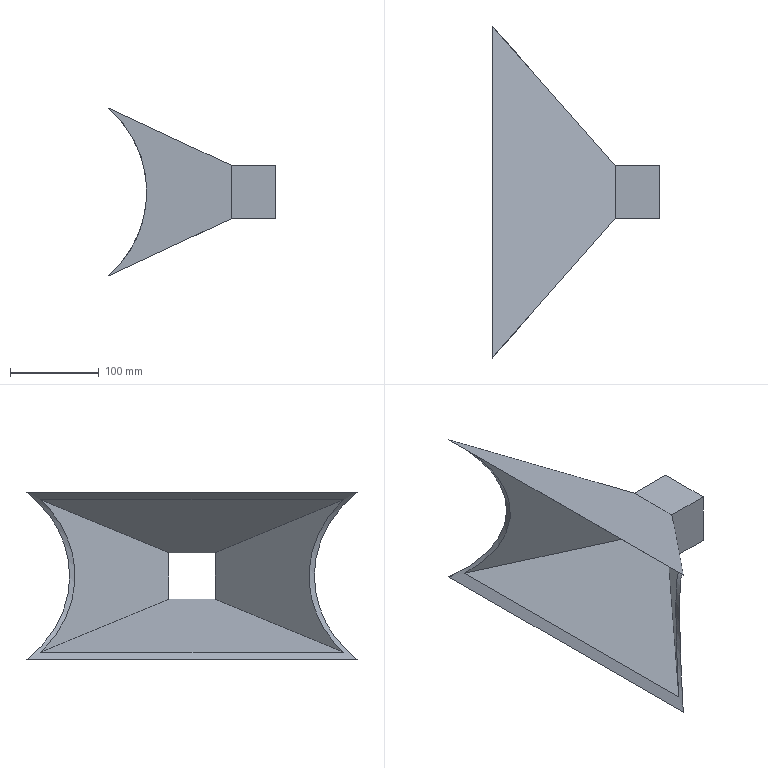Part | NX | features NSIDED_SURFACE 6, DATUM_CSYS 5, LINE 4, SKETCH 3, EXTRUDE 2, SEW 1, SHELL 1 | 1 solid | 18 faces | box 188.137 x 373.11 x 188.928 mm | volume 418507 mm3 | spline 9 | plane 8 | cylinder 1 | commonest cylinder face diameters 250 x1
STEP:
#1=CARTESIAN_POINT('',(11.863,-186.555,94.464));
#2=VERTEX_POINT('',#1);
#3=CARTESIAN_POINT('',(11.863,186.555,94.464));
#4=VERTEX_POINT('',#3);
#5=CARTESIAN_POINT('',(11.863,-186.555,94.464));
#6=CARTESIAN_POINT('',(11.863,-62.185,94.464));
#7=CARTESIAN_POINT('',(11.863,62.185,94.464));
#8=CARTESIAN_POINT('',(11.863,186.555,94.464));
#9=B_SPLINE_CURVE_WITH_KNOTS('',3,(#5,#6,#7,#8),.UNSPECIFIED.,.F.,.F.,(4,4),(0.02059,0.3937),.UNSPECIFIED.);
#10=EDGE_CURVE('',#2,#4,#9,.T.);
#11=ORIENTED_EDGE('',*,*,#10,.F.);
#12=CARTESIAN_POINT('',(150.,-30.,30.));
#13=VERTEX_POINT('',#12);
#14=CARTESIAN_POINT('',(150.,-30.,30.));
#15=CARTESIAN_POINT('',(103.954,-82.185,51.488));
#16=CARTESIAN_POINT('',(57.909,-134.37,72.976));
#17=CARTESIAN_POINT('',(11.863,-186.555,94.464));
#18=B_SPLINE_CURVE_WITH_KNOTS('',3,(#14,#15,#16,#17),.UNSPECIFIED.,.F.,.F.,(4,4),(0.,0.9209),.UNSPECIFIED.);
#19=EDGE_CURVE('',#2,#13,#18,.F.);
#20=ORIENTED_EDGE('',*,*,#19,.T.);
#21=CARTESIAN_POINT('',(150.,30.,30.));
#22=VERTEX_POINT('',#21);
#23=CARTESIAN_POINT('',(150.,-30.,30.));
#24=CARTESIAN_POINT('',(150.,-10.,30.));
#25=CARTESIAN_POINT('',(150.,10.,30.));
#26=CARTESIAN_POINT('',(150.,30.,30.));
#27=B_SPLINE_CURVE_WITH_KNOTS('',3,(#23,#24,#25,#26),.UNSPECIFIED.,.F.,.F.,(4,4),(0.,1.),.UNSPECIFIED.);
#28=EDGE_CURVE('',#22,#13,#27,.F.);
#29=ORIENTED_EDGE('',*,*,#28,.F.);
#30=CARTESIAN_POINT('',(11.863,186.555,94.464));
#31=CARTESIAN_POINT('',(57.909,134.37,72.976));
#32=CARTESIAN_POINT('',(103.954,82.185,51.488));
#33=CARTESIAN_POINT('',(150.,30.,30.));
#34=B_SPLINE_CURVE_WITH_KNOTS('',3,(#30,#31,#32,#33),.UNSPECIFIED.,.F.,.F.,(4,4),(0.07909,1.),.UNSPECIFIED.);
#35=EDGE_CURVE('',#22,#4,#34,.F.);
#36=ORIENTED_EDGE('',*,*,#35,.T.);
#37=EDGE_LOOP('',(#11,#20,#29,#36));
#38=FACE_BOUND('',#37,.T.);
#39=CARTESIAN_POINT('',(198.589,114.103,7.325));
#40=CARTESIAN_POINT('',(136.194,139.062,36.443));
#41=CARTESIAN_POINT('',(73.799,164.02,65.561));
#42=CARTESIAN_POINT('',(11.403,188.978,94.678));
#43=CARTESIAN_POINT('',(162.048,2.857,24.378));
#44=CARTESIAN_POINT('',(99.653,27.815,53.495));
#45=CARTESIAN_POINT('',(37.258,52.773,82.613));
#46=CARTESIAN_POINT('',(-25.137,77.731,111.731));
#47=CARTESIAN_POINT('',(125.507,-108.389,41.43));
#48=CARTESIAN_POINT('',(63.112,-83.431,70.548));
#49=CARTESIAN_POINT('',(0.7171,-58.473,99.665));
#50=CARTESIAN_POINT('',(-61.678,-33.515,128.783));
#51=CARTESIAN_POINT('',(88.967,-219.635,58.482));
#52=CARTESIAN_POINT('',(26.572,-194.677,87.6));
#53=CARTESIAN_POINT('',(-35.824,-169.719,116.718));
#54=CARTESIAN_POINT('',(-98.219,-144.761,145.835));
#55=B_SPLINE_SURFACE_WITH_KNOTS('',3,3,((#39,#40,#41,#42),(#43,#44,#45,#46),(#47,#48,#49,#50),(#51,#52,#53,#54)),.PLANE_SURF.,.F.,.F.,.F.,(4,4),(4,4),(0.06014,0.9183),(0.04039,0.894),.PIECEWISE_BEZIER_KNOTS.);
#56=ADVANCED_FACE('',(#38),#55,.F.);
#57=CARTESIAN_POINT('',(11.863,186.555,-94.464));
#58=VERTEX_POINT('',#57);
#59=CARTESIAN_POINT('',(150.,30.,-30.));
#60=VERTEX_POINT('',#59);
#61=CARTESIAN_POINT('',(150.,30.,-30.));
#62=CARTESIAN_POINT('',(103.954,82.185,-51.488));
#63=CARTESIAN_POINT('',(57.909,134.37,-72.976));
#64=CARTESIAN_POINT('',(11.863,186.555,-94.464));
#65=B_SPLINE_CURVE_WITH_KNOTS('',3,(#61,#62,#63,#64),.UNSPECIFIED.,.F.,.F.,(4,4),(0.,0.9209),.UNSPECIFIED.);
#66=EDGE_CURVE('',#58,#60,#65,.F.);
#67=ORIENTED_EDGE('',*,*,#66,.F.);
#68=CARTESIAN_POINT('',(11.863,186.555,-94.464));
#69=CARTESIAN_POINT('',(17.564,180.094,-89.523));
#70=CARTESIAN_POINT('',(25.67,170.908,-81.178));
#71=CARTESIAN_POINT('',(35.443,159.831,-67.546));
#72=CARTESIAN_POINT('',(41.976,152.427,-56.089));
#73=CARTESIAN_POINT('',(47.447,146.227,-43.563));
#74=CARTESIAN_POINT('',(51.699,141.408,-29.737));
#75=CARTESIAN_POINT('',(54.343,138.411,-15.433));
#76=CARTESIAN_POINT('',(55.306,137.32,-0.2027));
#77=CARTESIAN_POINT('',(54.431,138.312,14.717));
#78=CARTESIAN_POINT('',(51.777,141.32,29.447));
#79=CARTESIAN_POINT('',(47.611,146.041,43.117));
#80=CARTESIAN_POINT('',(40.246,154.388,60.121));
#81=CARTESIAN_POINT('',(31.021,164.843,74.408));
#82=CARTESIAN_POINT('',(20.354,176.932,86.652));
#83=CARTESIAN_POINT('',(14.74,183.294,91.97));
#84=CARTESIAN_POINT('',(11.863,186.555,94.464));
#85=B_SPLINE_CURVE_WITH_KNOTS('',3,(#68,#69,#70,#71,#72,#73,#74,#75,#76,#77,#78,#79,#80,#81,#82,#83,#84),.UNSPECIFIED.,.F.,.F.,(4,1,1,1,1,1,1,1,1,1,1,1,1,1,4),(0.01898,0.04869,0.06354,0.0784,0.09325,0.1081,0.123,0.1378,0.1527,0.1675,0.1824,0.1972,0.2269,0.2418,0.2566),.UNSPECIFIED.);
#86=EDGE_CURVE('',#4,#58,#85,.F.);
#87=ORIENTED_EDGE('',*,*,#86,.F.);
#88=ORIENTED_EDGE('',*,*,#35,.F.);
#89=CARTESIAN_POINT('',(150.,30.,30.));
#90=CARTESIAN_POINT('',(150.,30.,10.));
#91=CARTESIAN_POINT('',(150.,30.,-10.));
#92=CARTESIAN_POINT('',(150.,30.,-30.));
#93=B_SPLINE_CURVE_WITH_KNOTS('',3,(#89,#90,#91,#92),.UNSPECIFIED.,.F.,.F.,(4,4),(0.,1.),.UNSPECIFIED.);
#94=EDGE_CURVE('',#60,#22,#93,.F.);
#95=ORIENTED_EDGE('',*,*,#94,.F.);
#96=EDGE_LOOP('',(#67,#87,#88,#95));
#97=FACE_BOUND('',#96,.T.);
#98=CARTESIAN_POINT('',(-51.849,258.762,5.625));
#99=CARTESIAN_POINT('',(-16.061,218.203,-51.761));
#100=CARTESIAN_POINT('',(19.726,177.644,-109.148));
#101=CARTESIAN_POINT('',(55.514,137.084,-166.535));
#102=CARTESIAN_POINT('',(-13.308,215.083,60.532));
#103=CARTESIAN_POINT('',(22.479,174.523,3.145));
#104=CARTESIAN_POINT('',(58.267,133.964,-54.242));
#105=CARTESIAN_POINT('',(94.055,93.405,-111.629));
#106=CARTESIAN_POINT('',(25.233,171.403,115.438));
#107=CARTESIAN_POINT('',(61.02,130.844,58.051));
#108=CARTESIAN_POINT('',(96.808,90.285,0.664));
#109=CARTESIAN_POINT('',(132.595,49.725,-56.723));
#110=CARTESIAN_POINT('',(63.773,127.724,170.344));
#111=CARTESIAN_POINT('',(99.561,87.164,112.957));
#112=CARTESIAN_POINT('',(135.348,46.605,55.57));
#113=CARTESIAN_POINT('',(171.136,6.046,-1.817));
#114=B_SPLINE_SURFACE_WITH_KNOTS('',3,3,((#98,#99,#100,#101),(#102,#103,#104,#105),(#106,#107,#108,#109),(#110,#111,#112,#113)),.PLANE_SURF.,.F.,.F.,.F.,(4,4),(4,4),(0.1006,0.9596),(0.0997,0.9596),.PIECEWISE_BEZIER_KNOTS.);
#115=ADVANCED_FACE('',(#97),#114,.T.);
#116=ORIENTED_EDGE('',*,*,#19,.F.);
#117=CARTESIAN_POINT('',(11.863,-186.555,-94.464));
#118=VERTEX_POINT('',#117);
#119=CARTESIAN_POINT('',(11.863,-186.555,94.464));
#120=CARTESIAN_POINT('',(17.564,-180.094,89.523));
#121=CARTESIAN_POINT('',(25.67,-170.908,81.178));
#122=CARTESIAN_POINT('',(35.443,-159.831,67.546));
#123=CARTESIAN_POINT('',(41.976,-152.427,56.089));
#124=CARTESIAN_POINT('',(47.447,-146.227,43.563));
#125=CARTESIAN_POINT('',(51.699,-141.408,29.737));
#126=CARTESIAN_POINT('',(54.343,-138.411,15.433));
#127=CARTESIAN_POINT('',(55.306,-137.32,0.2027));
#128=CARTESIAN_POINT('',(54.431,-138.312,-14.717));
#129=CARTESIAN_POINT('',(51.777,-141.32,-29.447));
#130=CARTESIAN_POINT('',(47.611,-146.041,-43.117));
#131=CARTESIAN_POINT('',(40.246,-154.388,-60.121));
#132=CARTESIAN_POINT('',(31.021,-164.843,-74.408));
#133=CARTESIAN_POINT('',(20.354,-176.932,-86.652));
#134=CARTESIAN_POINT('',(14.74,-183.294,-91.97));
#135=CARTESIAN_POINT('',(11.863,-186.555,-94.464));
#136=B_SPLINE_CURVE_WITH_KNOTS('',3,(#119,#120,#121,#122,#123,#124,#125,#126,#127,#128,#129,#130,#131,#132,#133,#134,#135),.UNSPECIFIED.,.F.,.F.,(4,1,1,1,1,1,1,1,1,1,1,1,1,1,4),(0.01898,0.04869,0.06354,0.0784,0.09325,0.1081,0.123,0.1378,0.1527,0.1675,0.1824,0.1972,0.2269,0.2418,0.2566),.UNSPECIFIED.);
#137=EDGE_CURVE('',#118,#2,#136,.F.);
#138=ORIENTED_EDGE('',*,*,#137,.F.);
#139=CARTESIAN_POINT('',(150.,-30.,-30.));
#140=VERTEX_POINT('',#139);
#141=CARTESIAN_POINT('',(11.863,-186.555,-94.464));
#142=CARTESIAN_POINT('',(57.909,-134.37,-72.976));
#143=CARTESIAN_POINT('',(103.954,-82.185,-51.488));
#144=CARTESIAN_POINT('',(150.,-30.,-30.));
#145=B_SPLINE_CURVE_WITH_KNOTS('',3,(#141,#142,#143,#144),.UNSPECIFIED.,.F.,.F.,(4,4),(0.07909,1.),.UNSPECIFIED.);
#146=EDGE_CURVE('',#140,#118,#145,.F.);
#147=ORIENTED_EDGE('',*,*,#146,.F.);
#148=CARTESIAN_POINT('',(150.,-30.,-30.));
#149=CARTESIAN_POINT('',(150.,-30.,-10.));
#150=CARTESIAN_POINT('',(150.,-30.,10.));
#151=CARTESIAN_POINT('',(150.,-30.,30.));
#152=B_SPLINE_CURVE_WITH_KNOTS('',3,(#148,#149,#150,#151),.UNSPECIFIED.,.F.,.F.,(4,4),(0.,1.),.UNSPECIFIED.);
#153=EDGE_CURVE('',#13,#140,#152,.F.);
#154=ORIENTED_EDGE('',*,*,#153,.F.);
#155=EDGE_LOOP('',(#116,#138,#147,#154));
#156=FACE_BOUND('',#155,.T.);
#157=CARTESIAN_POINT('',(-51.849,-258.762,-5.625));
#158=CARTESIAN_POINT('',(-16.061,-218.203,51.761));
#159=CARTESIAN_POINT('',(19.726,-177.644,109.148));
#160=CARTESIAN_POINT('',(55.514,-137.084,166.535));
#161=CARTESIAN_POINT('',(-13.308,-215.083,-60.532));
#162=CARTESIAN_POINT('',(22.479,-174.523,-3.145));
#163=CARTESIAN_POINT('',(58.267,-133.964,54.242));
#164=CARTESIAN_POINT('',(94.055,-93.405,111.629));
#165=CARTESIAN_POINT('',(25.233,-171.403,-115.438));
#166=CARTESIAN_POINT('',(61.02,-130.844,-58.051));
#167=CARTESIAN_POINT('',(96.808,-90.285,-0.664));
#168=CARTESIAN_POINT('',(132.595,-49.725,56.723));
#169=CARTESIAN_POINT('',(63.773,-127.724,-170.344));
#170=CARTESIAN_POINT('',(99.561,-87.164,-112.957));
#171=CARTESIAN_POINT('',(135.348,-46.605,-55.57));
#172=CARTESIAN_POINT('',(171.136,-6.046,1.817));
#173=B_SPLINE_SURFACE_WITH_KNOTS('',3,3,((#157,#158,#159,#160),(#161,#162,#163,#164),(#165,#166,#167,#168),(#169,#170,#171,#172)),.PLANE_SURF.,.F.,.F.,.F.,(4,4),(4,4),(0.1006,0.9596),(0.0997,0.9596),.PIECEWISE_BEZIER_KNOTS.);
#174=ADVANCED_FACE('',(#156),#173,.T.);
#175=ORIENTED_EDGE('',*,*,#146,.T.);
#176=CARTESIAN_POINT('',(11.863,-186.555,-94.464));
#177=CARTESIAN_POINT('',(11.863,-62.185,-94.464));
#178=CARTESIAN_POINT('',(11.863,62.185,-94.464));
#179=CARTESIAN_POINT('',(11.863,186.555,-94.464));
#180=B_SPLINE_CURVE_WITH_KNOTS('',3,(#176,#177,#178,#179),.UNSPECIFIED.,.F.,.F.,(4,4),(0.0111,0.3842),.UNSPECIFIED.);
#181=EDGE_CURVE('',#118,#58,#180,.T.);
#182=ORIENTED_EDGE('',*,*,#181,.T.);
#183=ORIENTED_EDGE('',*,*,#66,.T.);
#184=CARTESIAN_POINT('',(150.,-30.,-30.));
#185=CARTESIAN_POINT('',(150.,-10.,-30.));
#186=CARTESIAN_POINT('',(150.,10.,-30.));
#187=CARTESIAN_POINT('',(150.,30.,-30.));
#188=B_SPLINE_CURVE_WITH_KNOTS('',3,(#184,#185,#186,#187),.UNSPECIFIED.,.F.,.F.,(4,4),(0.,1.),.UNSPECIFIED.);
#189=EDGE_CURVE('',#60,#140,#188,.F.);
#190=ORIENTED_EDGE('',*,*,#189,.T.);
#191=EDGE_LOOP('',(#175,#182,#183,#190));
#192=FACE_BOUND('',#191,.T.);
#193=CARTESIAN_POINT('',(88.967,219.635,-58.482));
#194=CARTESIAN_POINT('',(26.572,194.677,-87.6));
#195=CARTESIAN_POINT('',(-35.824,169.719,-116.718));
#196=CARTESIAN_POINT('',(-98.219,144.761,-145.835));
#197=CARTESIAN_POINT('',(125.507,108.389,-41.43));
#198=CARTESIAN_POINT('',(63.112,83.431,-70.548));
#199=CARTESIAN_POINT('',(0.7171,58.473,-99.665));
#200=CARTESIAN_POINT('',(-61.678,33.515,-128.783));
#201=CARTESIAN_POINT('',(162.048,-2.857,-24.378));
#202=CARTESIAN_POINT('',(99.653,-27.815,-53.495));
#203=CARTESIAN_POINT('',(37.258,-52.773,-82.613));
#204=CARTESIAN_POINT('',(-25.137,-77.731,-111.731));
#205=CARTESIAN_POINT('',(198.589,-114.103,-7.325));
#206=CARTESIAN_POINT('',(136.194,-139.062,-36.443));
#207=CARTESIAN_POINT('',(73.799,-164.02,-65.561));
#208=CARTESIAN_POINT('',(11.403,-188.978,-94.678));
#209=B_SPLINE_SURFACE_WITH_KNOTS('',3,3,((#193,#194,#195,#196),(#197,#198,#199,#200),(#201,#202,#203,#204),(#205,#206,#207,#208)),.PLANE_SURF.,.F.,.F.,.F.,(4,4),(4,4),(0.08171,0.9399),(0.04039,0.894),.PIECEWISE_BEZIER_KNOTS.);
#210=ADVANCED_FACE('',(#192),#209,.T.);
#211=CARTESIAN_POINT('',(20.85,-170.324,85.856));
#212=VERTEX_POINT('',#211);
#213=CARTESIAN_POINT('',(148.195,-26.,26.428));
#214=VERTEX_POINT('',#213);
#215=CARTESIAN_POINT('',(20.85,-170.324,85.856));
#216=CARTESIAN_POINT('',(63.299,-122.216,66.047));
#217=CARTESIAN_POINT('',(105.747,-74.108,46.237));
#218=CARTESIAN_POINT('',(148.195,-26.,26.428));
#219=B_SPLINE_CURVE_WITH_KNOTS('',3,(#215,#216,#217,#218),.UNSPECIFIED.,.F.,.F.,(4,4),(1.3,1.501),.UNSPECIFIED.);
#220=EDGE_CURVE('',#212,#214,#219,.T.);
#221=ORIENTED_EDGE('',*,*,#220,.F.);
#222=CARTESIAN_POINT('',(20.85,170.324,85.856));
#223=VERTEX_POINT('',#222);
#224=CARTESIAN_POINT('',(20.85,-170.324,85.856));
#225=CARTESIAN_POINT('',(20.85,-56.775,85.856));
#226=CARTESIAN_POINT('',(20.85,56.775,85.856));
#227=CARTESIAN_POINT('',(20.85,170.324,85.856));
#228=B_SPLINE_CURVE_WITH_KNOTS('',3,(#224,#225,#226,#227),.UNSPECIFIED.,.F.,.F.,(4,4),(0.0343,0.3749),.UNSPECIFIED.);
#229=EDGE_CURVE('',#212,#223,#228,.T.);
#230=ORIENTED_EDGE('',*,*,#229,.T.);
#231=CARTESIAN_POINT('',(148.195,26.,26.428));
#232=VERTEX_POINT('',#231);
#233=CARTESIAN_POINT('',(148.195,26.,26.428));
#234=CARTESIAN_POINT('',(105.747,74.108,46.237));
#235=CARTESIAN_POINT('',(63.299,122.216,66.047));
#236=CARTESIAN_POINT('',(20.85,170.324,85.856));
#237=B_SPLINE_CURVE_WITH_KNOTS('',3,(#233,#234,#235,#236),.UNSPECIFIED.,.F.,.F.,(4,4),(0.6508,0.8522),.UNSPECIFIED.);
#238=EDGE_CURVE('',#232,#223,#237,.T.);
#239=ORIENTED_EDGE('',*,*,#238,.F.);
#240=CARTESIAN_POINT('',(149.113,26.,26.));
#241=VERTEX_POINT('',#240);
#242=CARTESIAN_POINT('',(149.113,26.,26.));
#243=CARTESIAN_POINT('',(148.807,26.,26.143));
#244=CARTESIAN_POINT('',(148.501,26.,26.285));
#245=CARTESIAN_POINT('',(148.195,26.,26.428));
#246=B_SPLINE_CURVE_WITH_KNOTS('',3,(#242,#243,#244,#245),.UNSPECIFIED.,.F.,.F.,(4,4),(0.,0.001013),.UNSPECIFIED.);
#247=EDGE_CURVE('',#241,#232,#246,.T.);
#248=ORIENTED_EDGE('',*,*,#247,.F.);
#249=CARTESIAN_POINT('',(149.113,-26.,26.));
#250=VERTEX_POINT('',#249);
#251=CARTESIAN_POINT('',(149.113,26.,26.));
#252=CARTESIAN_POINT('',(149.113,8.667,26.));
#253=CARTESIAN_POINT('',(149.113,-8.667,26.));
#254=CARTESIAN_POINT('',(149.113,-26.,26.));
#255=B_SPLINE_CURVE_WITH_KNOTS('',3,(#251,#252,#253,#254),.UNSPECIFIED.,.F.,.F.,(4,4),(0.1439,0.1959),.UNSPECIFIED.);
#256=EDGE_CURVE('',#241,#250,#255,.T.);
#257=ORIENTED_EDGE('',*,*,#256,.T.);
#258=CARTESIAN_POINT('',(148.195,-26.,26.428));
#259=CARTESIAN_POINT('',(148.501,-26.,26.285));
#260=CARTESIAN_POINT('',(148.807,-26.,26.143));
#261=CARTESIAN_POINT('',(149.113,-26.,26.));
#262=B_SPLINE_CURVE_WITH_KNOTS('',3,(#258,#259,#260,#261),.UNSPECIFIED.,.F.,.F.,(4,4),(0.,0.001013),.UNSPECIFIED.);
#263=EDGE_CURVE('',#214,#250,#262,.T.);
#264=ORIENTED_EDGE('',*,*,#263,.F.);
#265=EDGE_LOOP('',(#221,#230,#239,#248,#257,#264));
#266=FACE_BOUND('',#265,.T.);
#267=CARTESIAN_POINT('',(192.83,103.576,5.598));
#268=CARTESIAN_POINT('',(135.361,126.563,32.417));
#269=CARTESIAN_POINT('',(77.891,149.551,59.237));
#270=CARTESIAN_POINT('',(20.422,172.539,86.056));
#271=CARTESIAN_POINT('',(159.469,2.008,21.167));
#272=CARTESIAN_POINT('',(101.999,24.996,47.986));
#273=CARTESIAN_POINT('',(44.53,47.984,74.805));
#274=CARTESIAN_POINT('',(-12.94,70.972,101.624));
#275=CARTESIAN_POINT('',(126.107,-99.559,36.736));
#276=CARTESIAN_POINT('',(68.638,-76.571,63.555));
#277=CARTESIAN_POINT('',(11.168,-53.583,90.374));
#278=CARTESIAN_POINT('',(-46.301,-30.595,117.193));
#279=CARTESIAN_POINT('',(92.746,-201.126,52.304));
#280=CARTESIAN_POINT('',(35.276,-178.138,79.124));
#281=CARTESIAN_POINT('',(-22.193,-155.15,105.943));
#282=CARTESIAN_POINT('',(-79.663,-132.162,132.762));
#283=B_SPLINE_SURFACE_WITH_KNOTS('',3,3,((#267,#268,#269,#270),(#271,#272,#273,#274),(#275,#276,#277,#278),(#279,#280,#281,#282)),.UNSPECIFIED.,.F.,.F.,.F.,(4,4),(4,4),(0.08776,0.8713),(0.04285,0.8291),.UNSPECIFIED.);
#284=ADVANCED_FACE('',(#266),#283,.T.);
#285=CARTESIAN_POINT('',(20.85,170.324,-85.856));
#286=VERTEX_POINT('',#285);
#287=CARTESIAN_POINT('',(20.85,170.324,-85.856));
#288=CARTESIAN_POINT('',(25.493,165.062,-80.943));
#289=CARTESIAN_POINT('',(32.083,157.594,-72.805));
#290=CARTESIAN_POINT('',(39.933,148.696,-59.865));
#291=CARTESIAN_POINT('',(45.023,142.928,-49.41));
#292=CARTESIAN_POINT('',(49.291,138.091,-38.03));
#293=CARTESIAN_POINT('',(52.517,134.434,-25.835));
#294=CARTESIAN_POINT('',(54.512,132.173,-13.323));
#295=CARTESIAN_POINT('',(55.231,131.36,-0.1538));
#296=CARTESIAN_POINT('',(54.564,132.115,12.821));
#297=CARTESIAN_POINT('',(52.581,134.363,25.569));
#298=CARTESIAN_POINT('',(49.367,138.005,37.783));
#299=CARTESIAN_POINT('',(45.134,142.802,49.162));
#300=CARTESIAN_POINT('',(39.982,148.641,59.774));
#301=CARTESIAN_POINT('',(34.2,155.195,69.335));
#302=CARTESIAN_POINT('',(27.827,162.417,78.056));
#303=CARTESIAN_POINT('',(23.212,167.647,83.357));
#304=CARTESIAN_POINT('',(20.85,170.324,85.856));
#305=B_SPLINE_CURVE_WITH_KNOTS('',3,(#287,#288,#289,#290,#291,#292,#293,#294,#295,#296,#297,#298,#299,#300,#301,#302,#303,#304),.UNSPECIFIED.,.F.,.F.,(4,1,1,1,1,1,1,1,1,1,1,1,1,1,1,4),(0.03181,0.0575,0.07035,0.0832,0.09605,0.1089,0.1217,0.1346,0.1474,0.1603,0.1731,0.186,0.1988,0.2117,0.2245,0.2374),.UNSPECIFIED.);
#306=EDGE_CURVE('',#223,#286,#305,.F.);
#307=ORIENTED_EDGE('',*,*,#306,.T.);
#308=CARTESIAN_POINT('',(148.195,26.,-26.428));
#309=VERTEX_POINT('',#308);
#310=CARTESIAN_POINT('',(20.85,170.324,-85.856));
#311=CARTESIAN_POINT('',(63.299,122.216,-66.047));
#312=CARTESIAN_POINT('',(105.747,74.108,-46.237));
#313=CARTESIAN_POINT('',(148.195,26.,-26.428));
#314=B_SPLINE_CURVE_WITH_KNOTS('',3,(#310,#311,#312,#313),.UNSPECIFIED.,.F.,.F.,(4,4),(1.3,1.501),.UNSPECIFIED.);
#315=EDGE_CURVE('',#286,#309,#314,.T.);
#316=ORIENTED_EDGE('',*,*,#315,.T.);
#317=CARTESIAN_POINT('',(148.195,26.,-26.428));
#318=CARTESIAN_POINT('',(148.195,26.,-8.809));
#319=CARTESIAN_POINT('',(148.195,26.,8.809));
#320=CARTESIAN_POINT('',(148.195,26.,26.428));
#321=B_SPLINE_CURVE_WITH_KNOTS('',3,(#317,#318,#319,#320),.UNSPECIFIED.,.F.,.F.,(4,4),(0.1434,0.1963),.UNSPECIFIED.);
#322=EDGE_CURVE('',#309,#232,#321,.T.);
#323=ORIENTED_EDGE('',*,*,#322,.T.);
#324=ORIENTED_EDGE('',*,*,#238,.T.);
#325=EDGE_LOOP('',(#307,#316,#323,#324));
#326=FACE_BOUND('',#325,.T.);
#327=CARTESIAN_POINT('',(-37.063,235.959,5.112));
#328=CARTESIAN_POINT('',(-4.345,198.879,-47.352));
#329=CARTESIAN_POINT('',(28.373,161.799,-99.817));
#330=CARTESIAN_POINT('',(61.091,124.718,-152.281));
#331=CARTESIAN_POINT('',(-1.807,196.002,55.339));
#332=CARTESIAN_POINT('',(30.911,158.922,2.875));
#333=CARTESIAN_POINT('',(63.629,121.842,-49.59));
#334=CARTESIAN_POINT('',(96.347,84.761,-102.055));
#335=CARTESIAN_POINT('',(33.449,156.046,105.566));
#336=CARTESIAN_POINT('',(66.167,118.965,53.101));
#337=CARTESIAN_POINT('',(98.885,81.885,0.6366));
#338=CARTESIAN_POINT('',(131.603,44.804,-51.828));
#339=CARTESIAN_POINT('',(68.705,116.089,155.793));
#340=CARTESIAN_POINT('',(101.423,79.008,103.328));
#341=CARTESIAN_POINT('',(134.141,41.928,50.863));
#342=CARTESIAN_POINT('',(166.859,4.847,-1.601));
#343=B_SPLINE_SURFACE_WITH_KNOTS('',3,3,((#327,#328,#329,#330),(#331,#332,#333,#334),(#335,#336,#337,#338),(#339,#340,#341,#342)),.UNSPECIFIED.,.F.,.F.,.F.,(4,4),(4,4),(0.1693,0.9551),(0.1681,0.9543),.UNSPECIFIED.);
#344=ADVANCED_FACE('',(#326),#343,.F.);
#345=CARTESIAN_POINT('',(20.85,-170.324,-85.856));
#346=VERTEX_POINT('',#345);
#347=CARTESIAN_POINT('',(20.85,-170.324,85.856));
#348=CARTESIAN_POINT('',(25.493,-165.062,80.943));
#349=CARTESIAN_POINT('',(32.083,-157.594,72.805));
#350=CARTESIAN_POINT('',(39.933,-148.696,59.865));
#351=CARTESIAN_POINT('',(45.023,-142.928,49.41));
#352=CARTESIAN_POINT('',(49.291,-138.091,38.03));
#353=CARTESIAN_POINT('',(52.517,-134.434,25.835));
#354=CARTESIAN_POINT('',(54.512,-132.173,13.323));
#355=CARTESIAN_POINT('',(55.231,-131.36,0.1538));
#356=CARTESIAN_POINT('',(54.564,-132.115,-12.821));
#357=CARTESIAN_POINT('',(52.581,-134.363,-25.569));
#358=CARTESIAN_POINT('',(49.367,-138.005,-37.783));
#359=CARTESIAN_POINT('',(45.134,-142.802,-49.162));
#360=CARTESIAN_POINT('',(39.982,-148.641,-59.774));
#361=CARTESIAN_POINT('',(34.2,-155.195,-69.335));
#362=CARTESIAN_POINT('',(27.827,-162.417,-78.056));
#363=CARTESIAN_POINT('',(23.212,-167.647,-83.357));
#364=CARTESIAN_POINT('',(20.85,-170.324,-85.856));
#365=B_SPLINE_CURVE_WITH_KNOTS('',3,(#347,#348,#349,#350,#351,#352,#353,#354,#355,#356,#357,#358,#359,#360,#361,#362,#363,#364),.UNSPECIFIED.,.F.,.F.,(4,1,1,1,1,1,1,1,1,1,1,1,1,1,1,4),(0.03181,0.0575,0.07035,0.0832,0.09605,0.1089,0.1217,0.1346,0.1474,0.1603,0.1731,0.186,0.1988,0.2117,0.2245,0.2374),.UNSPECIFIED.);
#366=EDGE_CURVE('',#346,#212,#365,.F.);
#367=ORIENTED_EDGE('',*,*,#366,.T.);
#368=ORIENTED_EDGE('',*,*,#220,.T.);
#369=CARTESIAN_POINT('',(148.195,-26.,-26.428));
#370=VERTEX_POINT('',#369);
#371=CARTESIAN_POINT('',(148.195,-26.,26.428));
#372=CARTESIAN_POINT('',(148.195,-26.,8.809));
#373=CARTESIAN_POINT('',(148.195,-26.,-8.809));
#374=CARTESIAN_POINT('',(148.195,-26.,-26.428));
#375=B_SPLINE_CURVE_WITH_KNOTS('',3,(#371,#372,#373,#374),.UNSPECIFIED.,.F.,.F.,(4,4),(0.1434,0.1963),.UNSPECIFIED.);
#376=EDGE_CURVE('',#214,#370,#375,.T.);
#377=ORIENTED_EDGE('',*,*,#376,.T.);
#378=CARTESIAN_POINT('',(148.195,-26.,-26.428));
#379=CARTESIAN_POINT('',(105.747,-74.108,-46.237));
#380=CARTESIAN_POINT('',(63.299,-122.216,-66.047));
#381=CARTESIAN_POINT('',(20.85,-170.324,-85.856));
#382=B_SPLINE_CURVE_WITH_KNOTS('',3,(#378,#379,#380,#381),.UNSPECIFIED.,.F.,.F.,(4,4),(0.6508,0.8522),.UNSPECIFIED.);
#383=EDGE_CURVE('',#370,#346,#382,.T.);
#384=ORIENTED_EDGE('',*,*,#383,.T.);
#385=EDGE_LOOP('',(#367,#368,#377,#384));
#386=FACE_BOUND('',#385,.T.);
#387=CARTESIAN_POINT('',(-37.063,-235.959,-5.112));
#388=CARTESIAN_POINT('',(-4.345,-198.879,47.352));
#389=CARTESIAN_POINT('',(28.373,-161.799,99.817));
#390=CARTESIAN_POINT('',(61.091,-124.718,152.281));
#391=CARTESIAN_POINT('',(-1.807,-196.002,-55.339));
#392=CARTESIAN_POINT('',(30.911,-158.922,-2.875));
#393=CARTESIAN_POINT('',(63.629,-121.842,49.59));
#394=CARTESIAN_POINT('',(96.347,-84.761,102.055));
#395=CARTESIAN_POINT('',(33.449,-156.046,-105.566));
#396=CARTESIAN_POINT('',(66.167,-118.965,-53.101));
#397=CARTESIAN_POINT('',(98.885,-81.885,-0.6366));
#398=CARTESIAN_POINT('',(131.603,-44.804,51.828));
#399=CARTESIAN_POINT('',(68.705,-116.089,-155.793));
#400=CARTESIAN_POINT('',(101.423,-79.008,-103.328));
#401=CARTESIAN_POINT('',(134.141,-41.928,-50.863));
#402=CARTESIAN_POINT('',(166.859,-4.847,1.601));
#403=B_SPLINE_SURFACE_WITH_KNOTS('',3,3,((#387,#388,#389,#390),(#391,#392,#393,#394),(#395,#396,#397,#398),(#399,#400,#401,#402)),.UNSPECIFIED.,.F.,.F.,.F.,(4,4),(4,4),(0.1693,0.9551),(0.1681,0.9543),.UNSPECIFIED.);
#404=ADVANCED_FACE('',(#386),#403,.F.);
#405=CARTESIAN_POINT('',(20.85,-170.324,-85.856));
#406=CARTESIAN_POINT('',(20.85,-56.775,-85.856));
#407=CARTESIAN_POINT('',(20.85,56.775,-85.856));
#408=CARTESIAN_POINT('',(20.85,170.324,-85.856));
#409=B_SPLINE_CURVE_WITH_KNOTS('',3,(#405,#406,#407,#408),.UNSPECIFIED.,.F.,.F.,(4,4),(0.01762,0.3583),.UNSPECIFIED.);
#410=EDGE_CURVE('',#346,#286,#409,.T.);
#411=ORIENTED_EDGE('',*,*,#410,.F.);
#412=ORIENTED_EDGE('',*,*,#383,.F.);
#413=CARTESIAN_POINT('',(149.113,-26.,-26.));
#414=VERTEX_POINT('',#413);
#415=CARTESIAN_POINT('',(149.113,-26.,-26.));
#416=CARTESIAN_POINT('',(148.807,-26.,-26.143));
#417=CARTESIAN_POINT('',(148.501,-26.,-26.285));
#418=CARTESIAN_POINT('',(148.195,-26.,-26.428));
#419=B_SPLINE_CURVE_WITH_KNOTS('',3,(#415,#416,#417,#418),.UNSPECIFIED.,.F.,.F.,(4,4),(0.,0.001013),.UNSPECIFIED.);
#420=EDGE_CURVE('',#414,#370,#419,.T.);
#421=ORIENTED_EDGE('',*,*,#420,.F.);
#422=CARTESIAN_POINT('',(149.113,26.,-26.));
#423=VERTEX_POINT('',#422);
#424=CARTESIAN_POINT('',(149.113,26.,-26.));
#425=CARTESIAN_POINT('',(149.113,8.667,-26.));
#426=CARTESIAN_POINT('',(149.113,-8.667,-26.));
#427=CARTESIAN_POINT('',(149.113,-26.,-26.));
#428=B_SPLINE_CURVE_WITH_KNOTS('',3,(#424,#425,#426,#427),.UNSPECIFIED.,.F.,.F.,(4,4),(0.1165,0.1685),.UNSPECIFIED.);
#429=EDGE_CURVE('',#423,#414,#428,.T.);
#430=ORIENTED_EDGE('',*,*,#429,.F.);
#431=CARTESIAN_POINT('',(148.195,26.,-26.428));
#432=CARTESIAN_POINT('',(148.501,26.,-26.285));
#433=CARTESIAN_POINT('',(148.807,26.,-26.143));
#434=CARTESIAN_POINT('',(149.113,26.,-26.));
#435=B_SPLINE_CURVE_WITH_KNOTS('',3,(#431,#432,#433,#434),.UNSPECIFIED.,.F.,.F.,(4,4),(0.,0.001013),.UNSPECIFIED.);
#436=EDGE_CURVE('',#309,#423,#435,.T.);
#437=ORIENTED_EDGE('',*,*,#436,.F.);
#438=ORIENTED_EDGE('',*,*,#315,.F.);
#439=EDGE_LOOP('',(#411,#412,#421,#430,#437,#438));
#440=FACE_BOUND('',#439,.T.);
#441=CARTESIAN_POINT('',(92.746,201.126,-52.304));
#442=CARTESIAN_POINT('',(35.276,178.138,-79.124));
#443=CARTESIAN_POINT('',(-22.193,155.15,-105.943));
#444=CARTESIAN_POINT('',(-79.663,132.162,-132.762));
#445=CARTESIAN_POINT('',(126.107,99.559,-36.736));
#446=CARTESIAN_POINT('',(68.638,76.571,-63.555));
#447=CARTESIAN_POINT('',(11.168,53.583,-90.374));
#448=CARTESIAN_POINT('',(-46.301,30.595,-117.193));
#449=CARTESIAN_POINT('',(159.469,-2.008,-21.167));
#450=CARTESIAN_POINT('',(101.999,-24.996,-47.986));
#451=CARTESIAN_POINT('',(44.53,-47.984,-74.805));
#452=CARTESIAN_POINT('',(-12.94,-70.972,-101.624));
#453=CARTESIAN_POINT('',(192.83,-103.576,-5.598));
#454=CARTESIAN_POINT('',(135.361,-126.563,-32.417));
#455=CARTESIAN_POINT('',(77.891,-149.551,-59.237));
#456=CARTESIAN_POINT('',(20.422,-172.539,-86.056));
#457=B_SPLINE_SURFACE_WITH_KNOTS('',3,3,((#441,#442,#443,#444),(#445,#446,#447,#448),(#449,#450,#451,#452),(#453,#454,#455,#456)),.UNSPECIFIED.,.F.,.F.,.F.,(4,4),(4,4),(0.1287,0.9122),(0.04285,0.8291),.UNSPECIFIED.);
#458=ADVANCED_FACE('',(#440),#457,.F.);
#459=ORIENTED_EDGE('',*,*,#94,.T.);
#460=CARTESIAN_POINT('',(200.,30.,30.));
#461=VERTEX_POINT('',#460);
#462=CARTESIAN_POINT('',(200.,30.,30.));
#463=DIRECTION('',(-1.,0.,0.));
#464=VECTOR('',#463,1000.);
#465=LINE('',#462,#464);
#466=EDGE_CURVE('',#461,#22,#465,.T.);
#467=ORIENTED_EDGE('',*,*,#466,.F.);
#468=CARTESIAN_POINT('',(200.,30.,-30.));
#469=VERTEX_POINT('',#468);
#470=CARTESIAN_POINT('',(200.,30.,30.));
#471=CARTESIAN_POINT('',(200.,30.,10.));
#472=CARTESIAN_POINT('',(200.,30.,-10.));
#473=CARTESIAN_POINT('',(200.,30.,-30.));
#474=B_SPLINE_CURVE_WITH_KNOTS('',3,(#470,#471,#472,#473),.UNSPECIFIED.,.F.,.F.,(4,4),(0.,1.),.UNSPECIFIED.);
#475=EDGE_CURVE('',#469,#461,#474,.F.);
#476=ORIENTED_EDGE('',*,*,#475,.F.);
#477=CARTESIAN_POINT('',(200.,30.,-30.));
#478=DIRECTION('',(-1.,0.,0.));
#479=VECTOR('',#478,1000.);
#480=LINE('',#477,#479);
#481=EDGE_CURVE('',#469,#60,#480,.T.);
#482=ORIENTED_EDGE('',*,*,#481,.T.);
#483=EDGE_LOOP('',(#459,#467,#476,#482));
#484=FACE_BOUND('',#483,.T.);
#485=CARTESIAN_POINT('',(200.,30.,-30.));
#486=DIRECTION('',(0.,-1.,0.));
#487=DIRECTION('',(0.,0.,-1.));
#488=AXIS2_PLACEMENT_3D('',#485,#486,#487);
#489=PLANE('',#488);
#490=ADVANCED_FACE('',(#484),#489,.F.);
#491=ORIENTED_EDGE('',*,*,#28,.T.);
#492=CARTESIAN_POINT('',(200.,-30.,30.));
#493=VERTEX_POINT('',#492);
#494=CARTESIAN_POINT('',(200.,-30.,30.));
#495=DIRECTION('',(-1.,0.,0.));
#496=VECTOR('',#495,1000.);
#497=LINE('',#494,#496);
#498=EDGE_CURVE('',#493,#13,#497,.T.);
#499=ORIENTED_EDGE('',*,*,#498,.F.);
#500=CARTESIAN_POINT('',(200.,-30.,30.));
#501=CARTESIAN_POINT('',(200.,-10.,30.));
#502=CARTESIAN_POINT('',(200.,10.,30.));
#503=CARTESIAN_POINT('',(200.,30.,30.));
#504=B_SPLINE_CURVE_WITH_KNOTS('',3,(#500,#501,#502,#503),.UNSPECIFIED.,.F.,.F.,(4,4),(0.,1.),.UNSPECIFIED.);
#505=EDGE_CURVE('',#461,#493,#504,.F.);
#506=ORIENTED_EDGE('',*,*,#505,.F.);
#507=ORIENTED_EDGE('',*,*,#466,.T.);
#508=EDGE_LOOP('',(#491,#499,#506,#507));
#509=FACE_BOUND('',#508,.T.);
#510=CARTESIAN_POINT('',(200.,30.,30.));
#511=DIRECTION('',(0.,0.,-1.));
#512=DIRECTION('',(0.,1.,0.));
#513=AXIS2_PLACEMENT_3D('',#510,#511,#512);
#514=PLANE('',#513);
#515=ADVANCED_FACE('',(#509),#514,.F.);
#516=ORIENTED_EDGE('',*,*,#153,.T.);
#517=CARTESIAN_POINT('',(200.,-30.,-30.));
#518=VERTEX_POINT('',#517);
#519=CARTESIAN_POINT('',(200.,-30.,-30.));
#520=DIRECTION('',(-1.,0.,0.));
#521=VECTOR('',#520,1000.);
#522=LINE('',#519,#521);
#523=EDGE_CURVE('',#518,#140,#522,.T.);
#524=ORIENTED_EDGE('',*,*,#523,.F.);
#525=CARTESIAN_POINT('',(200.,-30.,-30.));
#526=CARTESIAN_POINT('',(200.,-30.,-10.));
#527=CARTESIAN_POINT('',(200.,-30.,10.));
#528=CARTESIAN_POINT('',(200.,-30.,30.));
#529=B_SPLINE_CURVE_WITH_KNOTS('',3,(#525,#526,#527,#528),.UNSPECIFIED.,.F.,.F.,(4,4),(0.,1.),.UNSPECIFIED.);
#530=EDGE_CURVE('',#493,#518,#529,.F.);
#531=ORIENTED_EDGE('',*,*,#530,.F.);
#532=ORIENTED_EDGE('',*,*,#498,.T.);
#533=EDGE_LOOP('',(#516,#524,#531,#532));
#534=FACE_BOUND('',#533,.T.);
#535=CARTESIAN_POINT('',(200.,-30.,30.));
#536=DIRECTION('',(0.,1.,0.));
#537=DIRECTION('',(0.,0.,1.));
#538=AXIS2_PLACEMENT_3D('',#535,#536,#537);
#539=PLANE('',#538);
#540=ADVANCED_FACE('',(#534),#539,.F.);
#541=ORIENTED_EDGE('',*,*,#189,.F.);
#542=ORIENTED_EDGE('',*,*,#481,.F.);
#543=CARTESIAN_POINT('',(200.,-30.,-30.));
#544=CARTESIAN_POINT('',(200.,-10.,-30.));
#545=CARTESIAN_POINT('',(200.,10.,-30.));
#546=CARTESIAN_POINT('',(200.,30.,-30.));
#547=B_SPLINE_CURVE_WITH_KNOTS('',3,(#543,#544,#545,#546),.UNSPECIFIED.,.F.,.F.,(4,4),(0.,1.),.UNSPECIFIED.);
#548=EDGE_CURVE('',#469,#518,#547,.F.);
#549=ORIENTED_EDGE('',*,*,#548,.T.);
#550=ORIENTED_EDGE('',*,*,#523,.T.);
#551=EDGE_LOOP('',(#541,#542,#549,#550));
#552=FACE_BOUND('',#551,.T.);
#553=CARTESIAN_POINT('',(200.,30.,-30.));
#554=DIRECTION('',(0.,0.,-1.));
#555=DIRECTION('',(0.,1.,0.));
#556=AXIS2_PLACEMENT_3D('',#553,#554,#555);
#557=PLANE('',#556);
#558=ADVANCED_FACE('',(#552),#557,.T.);
#559=CARTESIAN_POINT('',(200.,26.,-26.));
#560=VERTEX_POINT('',#559);
#561=CARTESIAN_POINT('',(200.,26.,26.));
#562=VERTEX_POINT('',#561);
#563=CARTESIAN_POINT('',(200.,26.,-26.));
#564=CARTESIAN_POINT('',(200.,26.,-8.667));
#565=CARTESIAN_POINT('',(200.,26.,8.667));
#566=CARTESIAN_POINT('',(200.,26.,26.));
#567=B_SPLINE_CURVE_WITH_KNOTS('',3,(#563,#564,#565,#566),.UNSPECIFIED.,.F.,.F.,(4,4),(0.,0.052),.UNSPECIFIED.);
#568=EDGE_CURVE('',#560,#562,#567,.T.);
#569=ORIENTED_EDGE('',*,*,#568,.F.);
#570=CARTESIAN_POINT('',(200.,-26.,-26.));
#571=VERTEX_POINT('',#570);
#572=CARTESIAN_POINT('',(200.,26.,-26.));
#573=CARTESIAN_POINT('',(200.,8.667,-26.));
#574=CARTESIAN_POINT('',(200.,-8.667,-26.));
#575=CARTESIAN_POINT('',(200.,-26.,-26.));
#576=B_SPLINE_CURVE_WITH_KNOTS('',3,(#572,#573,#574,#575),.UNSPECIFIED.,.F.,.F.,(4,4),(0.,0.052),.UNSPECIFIED.);
#577=EDGE_CURVE('',#560,#571,#576,.T.);
#578=ORIENTED_EDGE('',*,*,#577,.T.);
#579=CARTESIAN_POINT('',(200.,-26.,26.));
#580=VERTEX_POINT('',#579);
#581=CARTESIAN_POINT('',(200.,-26.,26.));
#582=CARTESIAN_POINT('',(200.,-26.,8.667));
#583=CARTESIAN_POINT('',(200.,-26.,-8.667));
#584=CARTESIAN_POINT('',(200.,-26.,-26.));
#585=B_SPLINE_CURVE_WITH_KNOTS('',3,(#581,#582,#583,#584),.UNSPECIFIED.,.F.,.F.,(4,4),(0.,0.052),.UNSPECIFIED.);
#586=EDGE_CURVE('',#580,#571,#585,.T.);
#587=ORIENTED_EDGE('',*,*,#586,.F.);
#588=CARTESIAN_POINT('',(200.,26.,26.));
#589=CARTESIAN_POINT('',(200.,8.667,26.));
#590=CARTESIAN_POINT('',(200.,-8.667,26.));
#591=CARTESIAN_POINT('',(200.,-26.,26.));
#592=B_SPLINE_CURVE_WITH_KNOTS('',3,(#588,#589,#590,#591),.UNSPECIFIED.,.F.,.F.,(4,4),(0.,0.052),.UNSPECIFIED.);
#593=EDGE_CURVE('',#562,#580,#592,.T.);
#594=ORIENTED_EDGE('',*,*,#593,.F.);
#595=EDGE_LOOP('',(#569,#578,#587,#594));
#596=FACE_BOUND('',#595,.T.);
#597=ORIENTED_EDGE('',*,*,#475,.T.);
#598=ORIENTED_EDGE('',*,*,#505,.T.);
#599=ORIENTED_EDGE('',*,*,#530,.T.);
#600=ORIENTED_EDGE('',*,*,#548,.F.);
#601=EDGE_LOOP('',(#597,#598,#599,#600));
#602=FACE_BOUND('',#601,.T.);
#603=CARTESIAN_POINT('',(200.,-66.,0.));
#604=CARTESIAN_POINT('',(200.,-44.,22.));
#605=CARTESIAN_POINT('',(200.,-22.,44.));
#606=CARTESIAN_POINT('',(200.,0.,66.));
#607=CARTESIAN_POINT('',(200.,-44.,-22.));
#608=CARTESIAN_POINT('',(200.,-22.,0.));
#609=CARTESIAN_POINT('',(200.,0.,22.));
#610=CARTESIAN_POINT('',(200.,22.,44.));
#611=CARTESIAN_POINT('',(200.,-22.,-44.));
#612=CARTESIAN_POINT('',(200.,0.,-22.));
#613=CARTESIAN_POINT('',(200.,22.,0.));
#614=CARTESIAN_POINT('',(200.,44.,22.));
#615=CARTESIAN_POINT('',(200.,0.,-66.));
#616=CARTESIAN_POINT('',(200.,22.,-44.));
#617=CARTESIAN_POINT('',(200.,44.,-22.));
#618=CARTESIAN_POINT('',(200.,66.,0.));
#619=B_SPLINE_SURFACE_WITH_KNOTS('',3,3,((#603,#604,#605,#606),(#607,#608,#609,#610),(#611,#612,#613,#614),(#615,#616,#617,#618)),.PLANE_SURF.,.F.,.F.,.F.,(4,4),(4,4),(0.,1.),(0.,1.),.PIECEWISE_BEZIER_KNOTS.);
#620=ADVANCED_FACE('',(#596,#602),#619,.T.);
#621=ORIENTED_EDGE('',*,*,#322,.F.);
#622=ORIENTED_EDGE('',*,*,#436,.T.);
#623=CARTESIAN_POINT('',(200.,26.,-26.));
#624=DIRECTION('',(-1.,0.,0.));
#625=VECTOR('',#624,1000.);
#626=LINE('',#623,#625);
#627=EDGE_CURVE('',#560,#423,#626,.T.);
#628=ORIENTED_EDGE('',*,*,#627,.F.);
#629=ORIENTED_EDGE('',*,*,#568,.T.);
#630=CARTESIAN_POINT('',(200.,26.,26.));
#631=DIRECTION('',(-1.,0.,0.));
#632=VECTOR('',#631,1000.);
#633=LINE('',#630,#632);
#634=EDGE_CURVE('',#562,#241,#633,.T.);
#635=ORIENTED_EDGE('',*,*,#634,.T.);
#636=ORIENTED_EDGE('',*,*,#247,.T.);
#637=EDGE_LOOP('',(#621,#622,#628,#629,#635,#636));
#638=FACE_BOUND('',#637,.T.);
#639=CARTESIAN_POINT('',(200.,26.,-30.));
#640=DIRECTION('',(0.,-1.,0.));
#641=DIRECTION('',(0.,0.,-1.));
#642=AXIS2_PLACEMENT_3D('',#639,#640,#641);
#643=PLANE('',#642);
#644=ADVANCED_FACE('',(#638),#643,.T.);
#645=ORIENTED_EDGE('',*,*,#256,.F.);
#646=ORIENTED_EDGE('',*,*,#634,.F.);
#647=ORIENTED_EDGE('',*,*,#593,.T.);
#648=CARTESIAN_POINT('',(200.,-26.,26.));
#649=DIRECTION('',(-1.,0.,0.));
#650=VECTOR('',#649,1000.);
#651=LINE('',#648,#650);
#652=EDGE_CURVE('',#580,#250,#651,.T.);
#653=ORIENTED_EDGE('',*,*,#652,.T.);
#654=EDGE_LOOP('',(#645,#646,#647,#653));
#655=FACE_BOUND('',#654,.T.);
#656=CARTESIAN_POINT('',(200.,30.,26.));
#657=DIRECTION('',(0.,0.,-1.));
#658=DIRECTION('',(0.,1.,0.));
#659=AXIS2_PLACEMENT_3D('',#656,#657,#658);
#660=PLANE('',#659);
#661=ADVANCED_FACE('',(#655),#660,.T.);
#662=ORIENTED_EDGE('',*,*,#376,.F.);
#663=ORIENTED_EDGE('',*,*,#263,.T.);
#664=ORIENTED_EDGE('',*,*,#652,.F.);
#665=ORIENTED_EDGE('',*,*,#586,.T.);
#666=CARTESIAN_POINT('',(200.,-26.,-26.));
#667=DIRECTION('',(-1.,0.,0.));
#668=VECTOR('',#667,1000.);
#669=LINE('',#666,#668);
#670=EDGE_CURVE('',#571,#414,#669,.T.);
#671=ORIENTED_EDGE('',*,*,#670,.T.);
#672=ORIENTED_EDGE('',*,*,#420,.T.);
#673=EDGE_LOOP('',(#662,#663,#664,#665,#671,#672));
#674=FACE_BOUND('',#673,.T.);
#675=CARTESIAN_POINT('',(200.,-26.,30.));
#676=DIRECTION('',(0.,1.,0.));
#677=DIRECTION('',(0.,0.,1.));
#678=AXIS2_PLACEMENT_3D('',#675,#676,#677);
#679=PLANE('',#678);
#680=ADVANCED_FACE('',(#674),#679,.T.);
#681=ORIENTED_EDGE('',*,*,#429,.T.);
#682=ORIENTED_EDGE('',*,*,#670,.F.);
#683=ORIENTED_EDGE('',*,*,#577,.F.);
#684=ORIENTED_EDGE('',*,*,#627,.T.);
#685=EDGE_LOOP('',(#681,#682,#683,#684));
#686=FACE_BOUND('',#685,.T.);
#687=CARTESIAN_POINT('',(200.,30.,-26.));
#688=DIRECTION('',(0.,0.,-1.));
#689=DIRECTION('',(0.,1.,0.));
#690=AXIS2_PLACEMENT_3D('',#687,#688,#689);
#691=PLANE('',#690);
#692=ADVANCED_FACE('',(#686),#691,.F.);
#693=ORIENTED_EDGE('',*,*,#366,.F.);
#694=ORIENTED_EDGE('',*,*,#410,.T.);
#695=ORIENTED_EDGE('',*,*,#306,.F.);
#696=ORIENTED_EDGE('',*,*,#229,.F.);
#697=EDGE_LOOP('',(#693,#694,#695,#696));
#698=FACE_BOUND('',#697,.T.);
#699=ORIENTED_EDGE('',*,*,#10,.T.);
#700=ORIENTED_EDGE('',*,*,#86,.T.);
#701=ORIENTED_EDGE('',*,*,#181,.F.);
#702=ORIENTED_EDGE('',*,*,#137,.T.);
#703=EDGE_LOOP('',(#699,#700,#701,#702));
#704=FACE_BOUND('',#703,.T.);
#705=CARTESIAN_POINT('',(-70.,-220.,0.));
#706=DIRECTION('',(0.,1.,0.));
#707=DIRECTION('',(0.,0.,1.));
#708=AXIS2_PLACEMENT_3D('',#705,#706,#707);
#709=CYLINDRICAL_SURFACE('',#708,125.);
#710=ADVANCED_FACE('',(#698,#704),#709,.F.);
#711=CLOSED_SHELL('',(#56,#115,#174,#210,#284,#344,#404,#458,#490,#515,#540,#558,#620,#644,#661,#680,#692,#710));
#712=MANIFOLD_SOLID_BREP('',#711);
#713=(LENGTH_UNIT()NAMED_UNIT(*)SI_UNIT(.MILLI.,.METRE.));
#714=UNCERTAINTY_MEASURE_WITH_UNIT(LENGTH_MEASURE(0.0508),#713,'','');
#715=(NAMED_UNIT(*)PLANE_ANGLE_UNIT()SI_UNIT($,.RADIAN.));
#716=(NAMED_UNIT(*)SI_UNIT($,.STERADIAN.)SOLID_ANGLE_UNIT());
#717=(GEOMETRIC_REPRESENTATION_CONTEXT(3)GLOBAL_UNCERTAINTY_ASSIGNED_CONTEXT((#714))GLOBAL_UNIT_ASSIGNED_CONTEXT((#713,#715,#716))REPRESENTATION_CONTEXT('',''));
#718=ADVANCED_BREP_SHAPE_REPRESENTATION('',(#712),#717);